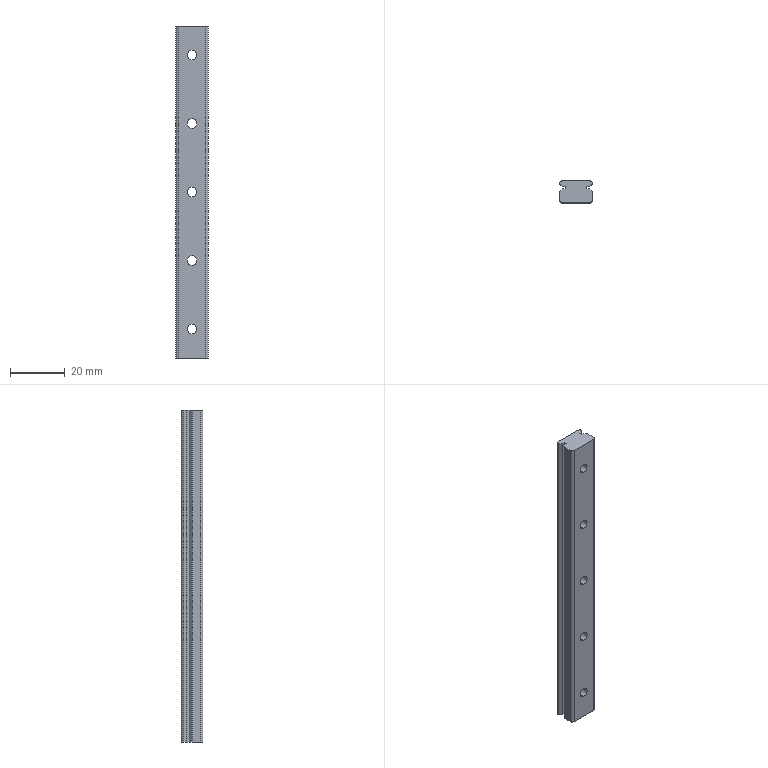Part | SolidWorks | features ICE 2, Extrusion 1 | 1 solid | 45 faces | box 12 x 8 x 121 mm | volume 9982 mm3 | cylinder 24 | plane 21 | commonest cylinder face diameters 3.5 x10 6 x10 2 x4
STEP:
#1=CARTESIAN_POINT('',(0.,-4.,108.75));
#2=VERTEX_POINT('',#1);
#3=CARTESIAN_POINT('',(0.,-4.,112.25));
#4=VERTEX_POINT('',#3);
#5=CARTESIAN_POINT('',(0.,-4.,110.5));
#6=DIRECTION('',(0.,1.,0.));
#7=DIRECTION('',(0.,0.,1.));
#8=AXIS2_PLACEMENT_3D('',#5,#6,#7);
#9=CIRCLE('',#8,1.75);
#10=EDGE_CURVE('',#2,#4,#9,.T.);
#11=ORIENTED_EDGE('',*,*,#10,.F.);
#12=CARTESIAN_POINT('',(0.,-0.5,108.75));
#13=VERTEX_POINT('',#12);
#14=CARTESIAN_POINT('',(0.,-4.,108.75));
#15=DIRECTION('',(0.,1.,0.));
#16=VECTOR('',#15,1000.);
#17=LINE('',#14,#16);
#18=EDGE_CURVE('',#2,#13,#17,.T.);
#19=ORIENTED_EDGE('',*,*,#18,.T.);
#20=CARTESIAN_POINT('',(0.,-0.5,112.25));
#21=VERTEX_POINT('',#20);
#22=CARTESIAN_POINT('',(0.,-0.5,110.5));
#23=DIRECTION('',(0.,1.,0.));
#24=DIRECTION('',(0.,0.,1.));
#25=AXIS2_PLACEMENT_3D('',#22,#23,#24);
#26=CIRCLE('',#25,1.75);
#27=EDGE_CURVE('',#13,#21,#26,.T.);
#28=ORIENTED_EDGE('',*,*,#27,.T.);
#29=CARTESIAN_POINT('',(0.,-4.,112.25));
#30=DIRECTION('',(0.,1.,0.));
#31=VECTOR('',#30,1000.);
#32=LINE('',#29,#31);
#33=EDGE_CURVE('',#4,#21,#32,.T.);
#34=ORIENTED_EDGE('',*,*,#33,.F.);
#35=EDGE_LOOP('',(#11,#19,#28,#34));
#36=FACE_OUTER_BOUND('',#35,.T.);
#37=CARTESIAN_POINT('',(0.,-4.,110.5));
#38=DIRECTION('',(0.,1.,0.));
#39=DIRECTION('',(0.,0.,1.));
#40=AXIS2_PLACEMENT_3D('',#37,#38,#39);
#41=CYLINDRICAL_SURFACE('',#40,1.75);
#42=ADVANCED_FACE('',(#36),#41,.F.);
#43=CARTESIAN_POINT('',(0.,-4.,83.75));
#44=VERTEX_POINT('',#43);
#45=CARTESIAN_POINT('',(0.,-4.,87.25));
#46=VERTEX_POINT('',#45);
#47=CARTESIAN_POINT('',(0.,-4.,85.5));
#48=DIRECTION('',(0.,1.,0.));
#49=DIRECTION('',(0.,0.,1.));
#50=AXIS2_PLACEMENT_3D('',#47,#48,#49);
#51=CIRCLE('',#50,1.75);
#52=EDGE_CURVE('',#44,#46,#51,.T.);
#53=ORIENTED_EDGE('',*,*,#52,.F.);
#54=CARTESIAN_POINT('',(0.,-0.5,83.75));
#55=VERTEX_POINT('',#54);
#56=CARTESIAN_POINT('',(0.,-4.,83.75));
#57=DIRECTION('',(0.,1.,0.));
#58=VECTOR('',#57,1000.);
#59=LINE('',#56,#58);
#60=EDGE_CURVE('',#44,#55,#59,.T.);
#61=ORIENTED_EDGE('',*,*,#60,.T.);
#62=CARTESIAN_POINT('',(0.,-0.5,87.25));
#63=VERTEX_POINT('',#62);
#64=CARTESIAN_POINT('',(0.,-0.5,85.5));
#65=DIRECTION('',(0.,1.,0.));
#66=DIRECTION('',(0.,0.,1.));
#67=AXIS2_PLACEMENT_3D('',#64,#65,#66);
#68=CIRCLE('',#67,1.75);
#69=EDGE_CURVE('',#55,#63,#68,.T.);
#70=ORIENTED_EDGE('',*,*,#69,.T.);
#71=CARTESIAN_POINT('',(0.,-4.,87.25));
#72=DIRECTION('',(0.,1.,0.));
#73=VECTOR('',#72,1000.);
#74=LINE('',#71,#73);
#75=EDGE_CURVE('',#46,#63,#74,.T.);
#76=ORIENTED_EDGE('',*,*,#75,.F.);
#77=EDGE_LOOP('',(#53,#61,#70,#76));
#78=FACE_OUTER_BOUND('',#77,.T.);
#79=CARTESIAN_POINT('',(0.,-4.,85.5));
#80=DIRECTION('',(0.,1.,0.));
#81=DIRECTION('',(0.,0.,1.));
#82=AXIS2_PLACEMENT_3D('',#79,#80,#81);
#83=CYLINDRICAL_SURFACE('',#82,1.75);
#84=ADVANCED_FACE('',(#78),#83,.F.);
#85=CARTESIAN_POINT('',(0.,-4.,58.75));
#86=VERTEX_POINT('',#85);
#87=CARTESIAN_POINT('',(0.,-4.,62.25));
#88=VERTEX_POINT('',#87);
#89=CARTESIAN_POINT('',(0.,-4.,60.5));
#90=DIRECTION('',(0.,1.,0.));
#91=DIRECTION('',(0.,0.,1.));
#92=AXIS2_PLACEMENT_3D('',#89,#90,#91);
#93=CIRCLE('',#92,1.75);
#94=EDGE_CURVE('',#86,#88,#93,.T.);
#95=ORIENTED_EDGE('',*,*,#94,.F.);
#96=CARTESIAN_POINT('',(0.,-0.5,58.75));
#97=VERTEX_POINT('',#96);
#98=CARTESIAN_POINT('',(0.,-4.,58.75));
#99=DIRECTION('',(0.,1.,0.));
#100=VECTOR('',#99,1000.);
#101=LINE('',#98,#100);
#102=EDGE_CURVE('',#86,#97,#101,.T.);
#103=ORIENTED_EDGE('',*,*,#102,.T.);
#104=CARTESIAN_POINT('',(0.,-0.5,62.25));
#105=VERTEX_POINT('',#104);
#106=CARTESIAN_POINT('',(0.,-0.5,60.5));
#107=DIRECTION('',(0.,1.,0.));
#108=DIRECTION('',(0.,0.,1.));
#109=AXIS2_PLACEMENT_3D('',#106,#107,#108);
#110=CIRCLE('',#109,1.75);
#111=EDGE_CURVE('',#97,#105,#110,.T.);
#112=ORIENTED_EDGE('',*,*,#111,.T.);
#113=CARTESIAN_POINT('',(0.,-4.,62.25));
#114=DIRECTION('',(0.,1.,0.));
#115=VECTOR('',#114,1000.);
#116=LINE('',#113,#115);
#117=EDGE_CURVE('',#88,#105,#116,.T.);
#118=ORIENTED_EDGE('',*,*,#117,.F.);
#119=EDGE_LOOP('',(#95,#103,#112,#118));
#120=FACE_OUTER_BOUND('',#119,.T.);
#121=CARTESIAN_POINT('',(0.,-4.,60.5));
#122=DIRECTION('',(0.,1.,0.));
#123=DIRECTION('',(0.,0.,1.));
#124=AXIS2_PLACEMENT_3D('',#121,#122,#123);
#125=CYLINDRICAL_SURFACE('',#124,1.75);
#126=ADVANCED_FACE('',(#120),#125,.F.);
#127=CARTESIAN_POINT('',(0.,-4.,8.75));
#128=VERTEX_POINT('',#127);
#129=CARTESIAN_POINT('',(0.,-4.,12.25));
#130=VERTEX_POINT('',#129);
#131=CARTESIAN_POINT('',(0.,-4.,10.5));
#132=DIRECTION('',(0.,1.,0.));
#133=DIRECTION('',(0.,0.,1.));
#134=AXIS2_PLACEMENT_3D('',#131,#132,#133);
#135=CIRCLE('',#134,1.75);
#136=EDGE_CURVE('',#128,#130,#135,.T.);
#137=ORIENTED_EDGE('',*,*,#136,.F.);
#138=CARTESIAN_POINT('',(0.,-0.5,8.75));
#139=VERTEX_POINT('',#138);
#140=CARTESIAN_POINT('',(0.,-4.,8.75));
#141=DIRECTION('',(0.,1.,0.));
#142=VECTOR('',#141,1000.);
#143=LINE('',#140,#142);
#144=EDGE_CURVE('',#128,#139,#143,.T.);
#145=ORIENTED_EDGE('',*,*,#144,.T.);
#146=CARTESIAN_POINT('',(0.,-0.5,12.25));
#147=VERTEX_POINT('',#146);
#148=CARTESIAN_POINT('',(0.,-0.5,10.5));
#149=DIRECTION('',(0.,1.,0.));
#150=DIRECTION('',(0.,0.,1.));
#151=AXIS2_PLACEMENT_3D('',#148,#149,#150);
#152=CIRCLE('',#151,1.75);
#153=EDGE_CURVE('',#139,#147,#152,.T.);
#154=ORIENTED_EDGE('',*,*,#153,.T.);
#155=CARTESIAN_POINT('',(0.,-4.,12.25));
#156=DIRECTION('',(0.,1.,0.));
#157=VECTOR('',#156,1000.);
#158=LINE('',#155,#157);
#159=EDGE_CURVE('',#130,#147,#158,.T.);
#160=ORIENTED_EDGE('',*,*,#159,.F.);
#161=EDGE_LOOP('',(#137,#145,#154,#160));
#162=FACE_OUTER_BOUND('',#161,.T.);
#163=CARTESIAN_POINT('',(0.,-4.,10.5));
#164=DIRECTION('',(0.,1.,0.));
#165=DIRECTION('',(0.,0.,1.));
#166=AXIS2_PLACEMENT_3D('',#163,#164,#165);
#167=CYLINDRICAL_SURFACE('',#166,1.75);
#168=ADVANCED_FACE('',(#162),#167,.F.);
#169=CARTESIAN_POINT('',(0.,-4.,33.75));
#170=VERTEX_POINT('',#169);
#171=CARTESIAN_POINT('',(0.,-4.,37.25));
#172=VERTEX_POINT('',#171);
#173=CARTESIAN_POINT('',(0.,-4.,35.5));
#174=DIRECTION('',(0.,1.,0.));
#175=DIRECTION('',(0.,0.,1.));
#176=AXIS2_PLACEMENT_3D('',#173,#174,#175);
#177=CIRCLE('',#176,1.75);
#178=EDGE_CURVE('',#170,#172,#177,.T.);
#179=ORIENTED_EDGE('',*,*,#178,.F.);
#180=CARTESIAN_POINT('',(0.,-0.5,33.75));
#181=VERTEX_POINT('',#180);
#182=CARTESIAN_POINT('',(0.,-4.,33.75));
#183=DIRECTION('',(0.,1.,0.));
#184=VECTOR('',#183,1000.);
#185=LINE('',#182,#184);
#186=EDGE_CURVE('',#170,#181,#185,.T.);
#187=ORIENTED_EDGE('',*,*,#186,.T.);
#188=CARTESIAN_POINT('',(0.,-0.5,37.25));
#189=VERTEX_POINT('',#188);
#190=CARTESIAN_POINT('',(0.,-0.5,35.5));
#191=DIRECTION('',(0.,1.,0.));
#192=DIRECTION('',(0.,0.,1.));
#193=AXIS2_PLACEMENT_3D('',#190,#191,#192);
#194=CIRCLE('',#193,1.75);
#195=EDGE_CURVE('',#181,#189,#194,.T.);
#196=ORIENTED_EDGE('',*,*,#195,.T.);
#197=CARTESIAN_POINT('',(0.,-4.,37.25));
#198=DIRECTION('',(0.,1.,0.));
#199=VECTOR('',#198,1000.);
#200=LINE('',#197,#199);
#201=EDGE_CURVE('',#172,#189,#200,.T.);
#202=ORIENTED_EDGE('',*,*,#201,.F.);
#203=EDGE_LOOP('',(#179,#187,#196,#202));
#204=FACE_OUTER_BOUND('',#203,.T.);
#205=CARTESIAN_POINT('',(0.,-4.,35.5));
#206=DIRECTION('',(0.,1.,0.));
#207=DIRECTION('',(0.,0.,1.));
#208=AXIS2_PLACEMENT_3D('',#205,#206,#207);
#209=CYLINDRICAL_SURFACE('',#208,1.75);
#210=ADVANCED_FACE('',(#204),#209,.F.);
#211=CARTESIAN_POINT('',(0.,-0.5,107.5));
#212=VERTEX_POINT('',#211);
#213=CARTESIAN_POINT('',(0.,-0.5,113.5));
#214=VERTEX_POINT('',#213);
#215=CARTESIAN_POINT('',(0.,-0.5,110.5));
#216=DIRECTION('',(0.,1.,0.));
#217=DIRECTION('',(0.,0.,1.));
#218=AXIS2_PLACEMENT_3D('',#215,#216,#217);
#219=CIRCLE('',#218,3.);
#220=EDGE_CURVE('',#212,#214,#219,.T.);
#221=ORIENTED_EDGE('',*,*,#220,.F.);
#222=CARTESIAN_POINT('',(0.,4.,107.5));
#223=VERTEX_POINT('',#222);
#224=CARTESIAN_POINT('',(0.,-0.5,107.5));
#225=DIRECTION('',(0.,1.,0.));
#226=VECTOR('',#225,1000.);
#227=LINE('',#224,#226);
#228=EDGE_CURVE('',#212,#223,#227,.T.);
#229=ORIENTED_EDGE('',*,*,#228,.T.);
#230=CARTESIAN_POINT('',(0.,4.,113.5));
#231=VERTEX_POINT('',#230);
#232=CARTESIAN_POINT('',(0.,4.,110.5));
#233=DIRECTION('',(0.,1.,0.));
#234=DIRECTION('',(0.,0.,1.));
#235=AXIS2_PLACEMENT_3D('',#232,#233,#234);
#236=CIRCLE('',#235,3.);
#237=EDGE_CURVE('',#223,#231,#236,.T.);
#238=ORIENTED_EDGE('',*,*,#237,.T.);
#239=CARTESIAN_POINT('',(0.,-0.5,113.5));
#240=DIRECTION('',(0.,1.,0.));
#241=VECTOR('',#240,1000.);
#242=LINE('',#239,#241);
#243=EDGE_CURVE('',#214,#231,#242,.T.);
#244=ORIENTED_EDGE('',*,*,#243,.F.);
#245=EDGE_LOOP('',(#221,#229,#238,#244));
#246=FACE_OUTER_BOUND('',#245,.T.);
#247=CARTESIAN_POINT('',(0.,-0.5,110.5));
#248=DIRECTION('',(0.,1.,0.));
#249=DIRECTION('',(0.,0.,1.));
#250=AXIS2_PLACEMENT_3D('',#247,#248,#249);
#251=CYLINDRICAL_SURFACE('',#250,3.);
#252=ADVANCED_FACE('',(#246),#251,.F.);
#253=CARTESIAN_POINT('',(0.,-0.5,82.5));
#254=VERTEX_POINT('',#253);
#255=CARTESIAN_POINT('',(0.,-0.5,88.5));
#256=VERTEX_POINT('',#255);
#257=CARTESIAN_POINT('',(0.,-0.5,85.5));
#258=DIRECTION('',(0.,1.,0.));
#259=DIRECTION('',(0.,0.,1.));
#260=AXIS2_PLACEMENT_3D('',#257,#258,#259);
#261=CIRCLE('',#260,3.);
#262=EDGE_CURVE('',#254,#256,#261,.T.);
#263=ORIENTED_EDGE('',*,*,#262,.F.);
#264=CARTESIAN_POINT('',(0.,4.,82.5));
#265=VERTEX_POINT('',#264);
#266=CARTESIAN_POINT('',(0.,-0.5,82.5));
#267=DIRECTION('',(0.,1.,0.));
#268=VECTOR('',#267,1000.);
#269=LINE('',#266,#268);
#270=EDGE_CURVE('',#254,#265,#269,.T.);
#271=ORIENTED_EDGE('',*,*,#270,.T.);
#272=CARTESIAN_POINT('',(0.,4.,88.5));
#273=VERTEX_POINT('',#272);
#274=CARTESIAN_POINT('',(0.,4.,85.5));
#275=DIRECTION('',(0.,1.,0.));
#276=DIRECTION('',(0.,0.,1.));
#277=AXIS2_PLACEMENT_3D('',#274,#275,#276);
#278=CIRCLE('',#277,3.);
#279=EDGE_CURVE('',#265,#273,#278,.T.);
#280=ORIENTED_EDGE('',*,*,#279,.T.);
#281=CARTESIAN_POINT('',(0.,-0.5,88.5));
#282=DIRECTION('',(0.,1.,0.));
#283=VECTOR('',#282,1000.);
#284=LINE('',#281,#283);
#285=EDGE_CURVE('',#256,#273,#284,.T.);
#286=ORIENTED_EDGE('',*,*,#285,.F.);
#287=EDGE_LOOP('',(#263,#271,#280,#286));
#288=FACE_OUTER_BOUND('',#287,.T.);
#289=CARTESIAN_POINT('',(0.,-0.5,85.5));
#290=DIRECTION('',(0.,1.,0.));
#291=DIRECTION('',(0.,0.,1.));
#292=AXIS2_PLACEMENT_3D('',#289,#290,#291);
#293=CYLINDRICAL_SURFACE('',#292,3.);
#294=ADVANCED_FACE('',(#288),#293,.F.);
#295=CARTESIAN_POINT('',(0.,-0.5,57.5));
#296=VERTEX_POINT('',#295);
#297=CARTESIAN_POINT('',(0.,-0.5,63.5));
#298=VERTEX_POINT('',#297);
#299=CARTESIAN_POINT('',(0.,-0.5,60.5));
#300=DIRECTION('',(0.,1.,0.));
#301=DIRECTION('',(0.,0.,1.));
#302=AXIS2_PLACEMENT_3D('',#299,#300,#301);
#303=CIRCLE('',#302,3.);
#304=EDGE_CURVE('',#296,#298,#303,.T.);
#305=ORIENTED_EDGE('',*,*,#304,.F.);
#306=CARTESIAN_POINT('',(0.,4.,57.5));
#307=VERTEX_POINT('',#306);
#308=CARTESIAN_POINT('',(0.,-0.5,57.5));
#309=DIRECTION('',(0.,1.,0.));
#310=VECTOR('',#309,1000.);
#311=LINE('',#308,#310);
#312=EDGE_CURVE('',#296,#307,#311,.T.);
#313=ORIENTED_EDGE('',*,*,#312,.T.);
#314=CARTESIAN_POINT('',(0.,4.,63.5));
#315=VERTEX_POINT('',#314);
#316=CARTESIAN_POINT('',(0.,4.,60.5));
#317=DIRECTION('',(0.,1.,0.));
#318=DIRECTION('',(0.,0.,1.));
#319=AXIS2_PLACEMENT_3D('',#316,#317,#318);
#320=CIRCLE('',#319,3.);
#321=EDGE_CURVE('',#307,#315,#320,.T.);
#322=ORIENTED_EDGE('',*,*,#321,.T.);
#323=CARTESIAN_POINT('',(0.,-0.5,63.5));
#324=DIRECTION('',(0.,1.,0.));
#325=VECTOR('',#324,1000.);
#326=LINE('',#323,#325);
#327=EDGE_CURVE('',#298,#315,#326,.T.);
#328=ORIENTED_EDGE('',*,*,#327,.F.);
#329=EDGE_LOOP('',(#305,#313,#322,#328));
#330=FACE_OUTER_BOUND('',#329,.T.);
#331=CARTESIAN_POINT('',(0.,-0.5,60.5));
#332=DIRECTION('',(0.,1.,0.));
#333=DIRECTION('',(0.,0.,1.));
#334=AXIS2_PLACEMENT_3D('',#331,#332,#333);
#335=CYLINDRICAL_SURFACE('',#334,3.);
#336=ADVANCED_FACE('',(#330),#335,.F.);
#337=CARTESIAN_POINT('',(0.,-0.5,32.5));
#338=VERTEX_POINT('',#337);
#339=CARTESIAN_POINT('',(0.,-0.5,38.5));
#340=VERTEX_POINT('',#339);
#341=CARTESIAN_POINT('',(0.,-0.5,35.5));
#342=DIRECTION('',(0.,1.,0.));
#343=DIRECTION('',(0.,0.,1.));
#344=AXIS2_PLACEMENT_3D('',#341,#342,#343);
#345=CIRCLE('',#344,3.);
#346=EDGE_CURVE('',#338,#340,#345,.T.);
#347=ORIENTED_EDGE('',*,*,#346,.F.);
#348=CARTESIAN_POINT('',(0.,4.,32.5));
#349=VERTEX_POINT('',#348);
#350=CARTESIAN_POINT('',(0.,-0.5,32.5));
#351=DIRECTION('',(0.,1.,0.));
#352=VECTOR('',#351,1000.);
#353=LINE('',#350,#352);
#354=EDGE_CURVE('',#338,#349,#353,.T.);
#355=ORIENTED_EDGE('',*,*,#354,.T.);
#356=CARTESIAN_POINT('',(0.,4.,38.5));
#357=VERTEX_POINT('',#356);
#358=CARTESIAN_POINT('',(0.,4.,35.5));
#359=DIRECTION('',(0.,1.,0.));
#360=DIRECTION('',(0.,0.,1.));
#361=AXIS2_PLACEMENT_3D('',#358,#359,#360);
#362=CIRCLE('',#361,3.);
#363=EDGE_CURVE('',#349,#357,#362,.T.);
#364=ORIENTED_EDGE('',*,*,#363,.T.);
#365=CARTESIAN_POINT('',(0.,-0.5,38.5));
#366=DIRECTION('',(0.,1.,0.));
#367=VECTOR('',#366,1000.);
#368=LINE('',#365,#367);
#369=EDGE_CURVE('',#340,#357,#368,.T.);
#370=ORIENTED_EDGE('',*,*,#369,.F.);
#371=EDGE_LOOP('',(#347,#355,#364,#370));
#372=FACE_OUTER_BOUND('',#371,.T.);
#373=CARTESIAN_POINT('',(0.,-0.5,35.5));
#374=DIRECTION('',(0.,1.,0.));
#375=DIRECTION('',(0.,0.,1.));
#376=AXIS2_PLACEMENT_3D('',#373,#374,#375);
#377=CYLINDRICAL_SURFACE('',#376,3.);
#378=ADVANCED_FACE('',(#372),#377,.F.);
#379=CARTESIAN_POINT('',(0.,-0.5,7.5));
#380=VERTEX_POINT('',#379);
#381=CARTESIAN_POINT('',(0.,-0.5,13.5));
#382=VERTEX_POINT('',#381);
#383=CARTESIAN_POINT('',(0.,-0.5,10.5));
#384=DIRECTION('',(0.,1.,0.));
#385=DIRECTION('',(0.,0.,1.));
#386=AXIS2_PLACEMENT_3D('',#383,#384,#385);
#387=CIRCLE('',#386,3.);
#388=EDGE_CURVE('',#380,#382,#387,.T.);
#389=ORIENTED_EDGE('',*,*,#388,.F.);
#390=CARTESIAN_POINT('',(0.,4.,7.5));
#391=VERTEX_POINT('',#390);
#392=CARTESIAN_POINT('',(0.,-0.5,7.5));
#393=DIRECTION('',(0.,1.,0.));
#394=VECTOR('',#393,1000.);
#395=LINE('',#392,#394);
#396=EDGE_CURVE('',#380,#391,#395,.T.);
#397=ORIENTED_EDGE('',*,*,#396,.T.);
#398=CARTESIAN_POINT('',(0.,4.,13.5));
#399=VERTEX_POINT('',#398);
#400=CARTESIAN_POINT('',(0.,4.,10.5));
#401=DIRECTION('',(0.,1.,0.));
#402=DIRECTION('',(0.,0.,1.));
#403=AXIS2_PLACEMENT_3D('',#400,#401,#402);
#404=CIRCLE('',#403,3.);
#405=EDGE_CURVE('',#391,#399,#404,.T.);
#406=ORIENTED_EDGE('',*,*,#405,.T.);
#407=CARTESIAN_POINT('',(0.,-0.5,13.5));
#408=DIRECTION('',(0.,1.,0.));
#409=VECTOR('',#408,1000.);
#410=LINE('',#407,#409);
#411=EDGE_CURVE('',#382,#399,#410,.T.);
#412=ORIENTED_EDGE('',*,*,#411,.F.);
#413=EDGE_LOOP('',(#389,#397,#406,#412));
#414=FACE_OUTER_BOUND('',#413,.T.);
#415=CARTESIAN_POINT('',(0.,-0.5,10.5));
#416=DIRECTION('',(0.,1.,0.));
#417=DIRECTION('',(0.,0.,1.));
#418=AXIS2_PLACEMENT_3D('',#415,#416,#417);
#419=CYLINDRICAL_SURFACE('',#418,3.);
#420=ADVANCED_FACE('',(#414),#419,.F.);
#421=CARTESIAN_POINT('',(-6.,-3.,0.));
#422=VERTEX_POINT('',#421);
#423=CARTESIAN_POINT('',(-5.,-4.,0.));
#424=VERTEX_POINT('',#423);
#425=CARTESIAN_POINT('',(-5.,-3.,0.));
#426=DIRECTION('',(0.,0.,1.));
#427=DIRECTION('',(1.,0.,0.));
#428=AXIS2_PLACEMENT_3D('',#425,#426,#427);
#429=CIRCLE('',#428,1.);
#430=EDGE_CURVE('',#422,#424,#429,.T.);
#431=ORIENTED_EDGE('',*,*,#430,.T.);
#432=CARTESIAN_POINT('',(-5.,-4.,121.));
#433=VERTEX_POINT('',#432);
#434=CARTESIAN_POINT('',(-5.,-4.,121.));
#435=DIRECTION('',(0.,0.,-1.));
#436=VECTOR('',#435,1000.);
#437=LINE('',#434,#436);
#438=EDGE_CURVE('',#433,#424,#437,.T.);
#439=ORIENTED_EDGE('',*,*,#438,.F.);
#440=CARTESIAN_POINT('',(-6.,-3.,121.));
#441=VERTEX_POINT('',#440);
#442=CARTESIAN_POINT('',(-5.,-3.,121.));
#443=DIRECTION('',(0.,0.,1.));
#444=DIRECTION('',(1.,0.,0.));
#445=AXIS2_PLACEMENT_3D('',#442,#443,#444);
#446=CIRCLE('',#445,1.);
#447=EDGE_CURVE('',#441,#433,#446,.T.);
#448=ORIENTED_EDGE('',*,*,#447,.F.);
#449=CARTESIAN_POINT('',(-6.,-3.,121.));
#450=DIRECTION('',(0.,0.,-1.));
#451=VECTOR('',#450,1000.);
#452=LINE('',#449,#451);
#453=EDGE_CURVE('',#441,#422,#452,.T.);
#454=ORIENTED_EDGE('',*,*,#453,.T.);
#455=EDGE_LOOP('',(#431,#439,#448,#454));
#456=FACE_OUTER_BOUND('',#455,.T.);
#457=CARTESIAN_POINT('',(-5.,-3.,121.));
#458=DIRECTION('',(0.,0.,-1.));
#459=DIRECTION('',(-1.,0.,0.));
#460=AXIS2_PLACEMENT_3D('',#457,#458,#459);
#461=CYLINDRICAL_SURFACE('',#460,1.);
#462=ADVANCED_FACE('',(#456),#461,.T.);
#463=CARTESIAN_POINT('',(0.,-4.,110.5));
#464=DIRECTION('',(0.,1.,0.));
#465=DIRECTION('',(0.,0.,1.));
#466=AXIS2_PLACEMENT_3D('',#463,#464,#465);
#467=CIRCLE('',#466,1.75);
#468=EDGE_CURVE('',#4,#2,#467,.T.);
#469=ORIENTED_EDGE('',*,*,#468,.T.);
#470=ORIENTED_EDGE('',*,*,#10,.T.);
#471=EDGE_LOOP('',(#469,#470));
#472=FACE_BOUND('',#471,.T.);
#473=CARTESIAN_POINT('',(0.,-4.,85.5));
#474=DIRECTION('',(0.,1.,0.));
#475=DIRECTION('',(0.,0.,1.));
#476=AXIS2_PLACEMENT_3D('',#473,#474,#475);
#477=CIRCLE('',#476,1.75);
#478=EDGE_CURVE('',#46,#44,#477,.T.);
#479=ORIENTED_EDGE('',*,*,#478,.T.);
#480=ORIENTED_EDGE('',*,*,#52,.T.);
#481=EDGE_LOOP('',(#479,#480));
#482=FACE_BOUND('',#481,.T.);
#483=CARTESIAN_POINT('',(0.,-4.,60.5));
#484=DIRECTION('',(0.,1.,0.));
#485=DIRECTION('',(0.,0.,1.));
#486=AXIS2_PLACEMENT_3D('',#483,#484,#485);
#487=CIRCLE('',#486,1.75);
#488=EDGE_CURVE('',#88,#86,#487,.T.);
#489=ORIENTED_EDGE('',*,*,#488,.T.);
#490=ORIENTED_EDGE('',*,*,#94,.T.);
#491=EDGE_LOOP('',(#489,#490));
#492=FACE_BOUND('',#491,.T.);
#493=CARTESIAN_POINT('',(0.,-4.,10.5));
#494=DIRECTION('',(0.,1.,0.));
#495=DIRECTION('',(0.,0.,1.));
#496=AXIS2_PLACEMENT_3D('',#493,#494,#495);
#497=CIRCLE('',#496,1.75);
#498=EDGE_CURVE('',#130,#128,#497,.T.);
#499=ORIENTED_EDGE('',*,*,#498,.T.);
#500=ORIENTED_EDGE('',*,*,#136,.T.);
#501=EDGE_LOOP('',(#499,#500));
#502=FACE_BOUND('',#501,.T.);
#503=CARTESIAN_POINT('',(0.,-4.,35.5));
#504=DIRECTION('',(0.,1.,0.));
#505=DIRECTION('',(0.,0.,1.));
#506=AXIS2_PLACEMENT_3D('',#503,#504,#505);
#507=CIRCLE('',#506,1.75);
#508=EDGE_CURVE('',#172,#170,#507,.T.);
#509=ORIENTED_EDGE('',*,*,#508,.T.);
#510=ORIENTED_EDGE('',*,*,#178,.T.);
#511=EDGE_LOOP('',(#509,#510));
#512=FACE_BOUND('',#511,.T.);
#513=CARTESIAN_POINT('',(5.,-4.,0.));
#514=VERTEX_POINT('',#513);
#515=CARTESIAN_POINT('',(-5.,-4.,0.));
#516=DIRECTION('',(1.,0.,0.));
#517=VECTOR('',#516,1000.);
#518=LINE('',#515,#517);
#519=EDGE_CURVE('',#424,#514,#518,.T.);
#520=ORIENTED_EDGE('',*,*,#519,.T.);
#521=CARTESIAN_POINT('',(5.,-4.,121.));
#522=VERTEX_POINT('',#521);
#523=CARTESIAN_POINT('',(5.,-4.,121.));
#524=DIRECTION('',(0.,0.,-1.));
#525=VECTOR('',#524,1000.);
#526=LINE('',#523,#525);
#527=EDGE_CURVE('',#522,#514,#526,.T.);
#528=ORIENTED_EDGE('',*,*,#527,.F.);
#529=CARTESIAN_POINT('',(-5.,-4.,121.));
#530=DIRECTION('',(1.,0.,0.));
#531=VECTOR('',#530,1000.);
#532=LINE('',#529,#531);
#533=EDGE_CURVE('',#433,#522,#532,.T.);
#534=ORIENTED_EDGE('',*,*,#533,.F.);
#535=ORIENTED_EDGE('',*,*,#438,.T.);
#536=EDGE_LOOP('',(#520,#528,#534,#535));
#537=FACE_OUTER_BOUND('',#536,.T.);
#538=CARTESIAN_POINT('',(-5.,-4.,121.));
#539=DIRECTION('',(0.,1.,0.));
#540=DIRECTION('',(0.,0.,1.));
#541=AXIS2_PLACEMENT_3D('',#538,#539,#540);
#542=PLANE('',#541);
#543=ADVANCED_FACE('',(#472,#482,#492,#502,#512,#537),#542,.F.);
#544=CARTESIAN_POINT('',(6.,-3.,0.));
#545=VERTEX_POINT('',#544);
#546=CARTESIAN_POINT('',(5.,-3.,0.));
#547=DIRECTION('',(0.,0.,1.));
#548=DIRECTION('',(1.,0.,0.));
#549=AXIS2_PLACEMENT_3D('',#546,#547,#548);
#550=CIRCLE('',#549,1.);
#551=EDGE_CURVE('',#514,#545,#550,.T.);
#552=ORIENTED_EDGE('',*,*,#551,.T.);
#553=CARTESIAN_POINT('',(6.,-3.,121.));
#554=VERTEX_POINT('',#553);
#555=CARTESIAN_POINT('',(6.,-3.,121.));
#556=DIRECTION('',(0.,0.,-1.));
#557=VECTOR('',#556,1000.);
#558=LINE('',#555,#557);
#559=EDGE_CURVE('',#554,#545,#558,.T.);
#560=ORIENTED_EDGE('',*,*,#559,.F.);
#561=CARTESIAN_POINT('',(5.,-3.,121.));
#562=DIRECTION('',(0.,0.,1.));
#563=DIRECTION('',(1.,0.,0.));
#564=AXIS2_PLACEMENT_3D('',#561,#562,#563);
#565=CIRCLE('',#564,1.);
#566=EDGE_CURVE('',#522,#554,#565,.T.);
#567=ORIENTED_EDGE('',*,*,#566,.F.);
#568=ORIENTED_EDGE('',*,*,#527,.T.);
#569=EDGE_LOOP('',(#552,#560,#567,#568));
#570=FACE_OUTER_BOUND('',#569,.T.);
#571=CARTESIAN_POINT('',(5.,-3.,121.));
#572=DIRECTION('',(0.,0.,-1.));
#573=DIRECTION('',(-1.,0.,0.));
#574=AXIS2_PLACEMENT_3D('',#571,#572,#573);
#575=CYLINDRICAL_SURFACE('',#574,1.);
#576=ADVANCED_FACE('',(#570),#575,.T.);
#577=CARTESIAN_POINT('',(6.,0.,0.));
#578=VERTEX_POINT('',#577);
#579=CARTESIAN_POINT('',(6.,0.,0.));
#580=DIRECTION('',(0.,1.,0.));
#581=VECTOR('',#580,1000.);
#582=LINE('',#579,#581);
#583=EDGE_CURVE('',#545,#578,#582,.T.);
#584=ORIENTED_EDGE('',*,*,#583,.T.);
#585=CARTESIAN_POINT('',(6.,0.,121.));
#586=VERTEX_POINT('',#585);
#587=CARTESIAN_POINT('',(6.,0.,121.));
#588=DIRECTION('',(0.,0.,-1.));
#589=VECTOR('',#588,1000.);
#590=LINE('',#587,#589);
#591=EDGE_CURVE('',#586,#578,#590,.T.);
#592=ORIENTED_EDGE('',*,*,#591,.F.);
#593=CARTESIAN_POINT('',(6.,0.,121.));
#594=DIRECTION('',(0.,1.,0.));
#595=VECTOR('',#594,1000.);
#596=LINE('',#593,#595);
#597=EDGE_CURVE('',#554,#586,#596,.T.);
#598=ORIENTED_EDGE('',*,*,#597,.F.);
#599=ORIENTED_EDGE('',*,*,#559,.T.);
#600=EDGE_LOOP('',(#584,#592,#598,#599));
#601=FACE_OUTER_BOUND('',#600,.T.);
#602=CARTESIAN_POINT('',(6.,0.,121.));
#603=DIRECTION('',(-1.,0.,0.));
#604=DIRECTION('',(0.,-1.,0.));
#605=AXIS2_PLACEMENT_3D('',#602,#603,#604);
#606=PLANE('',#605);
#607=ADVANCED_FACE('',(#601),#606,.F.);
#608=CARTESIAN_POINT('',(5.,1.,0.));
#609=VERTEX_POINT('',#608);
#610=CARTESIAN_POINT('',(5.,1.,0.));
#611=DIRECTION('',(-0.7071,0.7071,0.));
#612=VECTOR('',#611,1000.);
#613=LINE('',#610,#612);
#614=EDGE_CURVE('',#578,#609,#613,.T.);
#615=ORIENTED_EDGE('',*,*,#614,.T.);
#616=CARTESIAN_POINT('',(5.,1.,121.));
#617=VERTEX_POINT('',#616);
#618=CARTESIAN_POINT('',(5.,1.,121.));
#619=DIRECTION('',(0.,0.,-1.));
#620=VECTOR('',#619,1000.);
#621=LINE('',#618,#620);
#622=EDGE_CURVE('',#617,#609,#621,.T.);
#623=ORIENTED_EDGE('',*,*,#622,.F.);
#624=CARTESIAN_POINT('',(5.,1.,121.));
#625=DIRECTION('',(-0.7071,0.7071,0.));
#626=VECTOR('',#625,1000.);
#627=LINE('',#624,#626);
#628=EDGE_CURVE('',#586,#617,#627,.T.);
#629=ORIENTED_EDGE('',*,*,#628,.F.);
#630=ORIENTED_EDGE('',*,*,#591,.T.);
#631=EDGE_LOOP('',(#615,#623,#629,#630));
#632=FACE_OUTER_BOUND('',#631,.T.);
#633=CARTESIAN_POINT('',(5.,1.,121.));
#634=DIRECTION('',(-0.7071,-0.7071,0.));
#635=DIRECTION('',(0.7071,-0.7071,0.));
#636=AXIS2_PLACEMENT_3D('',#633,#634,#635);
#637=PLANE('',#636);
#638=ADVANCED_FACE('',(#632),#637,.F.);
#639=CARTESIAN_POINT('',(4.,1.,0.));
#640=VERTEX_POINT('',#639);
#641=CARTESIAN_POINT('',(4.,1.,0.));
#642=DIRECTION('',(-1.,0.,0.));
#643=VECTOR('',#642,1000.);
#644=LINE('',#641,#643);
#645=EDGE_CURVE('',#609,#640,#644,.T.);
#646=ORIENTED_EDGE('',*,*,#645,.T.);
#647=CARTESIAN_POINT('',(4.,1.,121.));
#648=VERTEX_POINT('',#647);
#649=CARTESIAN_POINT('',(4.,1.,121.));
#650=DIRECTION('',(0.,0.,-1.));
#651=VECTOR('',#650,1000.);
#652=LINE('',#649,#651);
#653=EDGE_CURVE('',#648,#640,#652,.T.);
#654=ORIENTED_EDGE('',*,*,#653,.F.);
#655=CARTESIAN_POINT('',(4.,1.,121.));
#656=DIRECTION('',(-1.,0.,0.));
#657=VECTOR('',#656,1000.);
#658=LINE('',#655,#657);
#659=EDGE_CURVE('',#617,#648,#658,.T.);
#660=ORIENTED_EDGE('',*,*,#659,.F.);
#661=ORIENTED_EDGE('',*,*,#622,.T.);
#662=EDGE_LOOP('',(#646,#654,#660,#661));
#663=FACE_OUTER_BOUND('',#662,.T.);
#664=CARTESIAN_POINT('',(4.,1.,121.));
#665=DIRECTION('',(0.,-1.,0.));
#666=DIRECTION('',(0.,0.,-1.));
#667=AXIS2_PLACEMENT_3D('',#664,#665,#666);
#668=PLANE('',#667);
#669=ADVANCED_FACE('',(#663),#668,.F.);
#670=CARTESIAN_POINT('',(4.,2.,0.));
#671=VERTEX_POINT('',#670);
#672=CARTESIAN_POINT('',(4.,2.,0.));
#673=DIRECTION('',(0.,1.,0.));
#674=VECTOR('',#673,1000.);
#675=LINE('',#672,#674);
#676=EDGE_CURVE('',#640,#671,#675,.T.);
#677=ORIENTED_EDGE('',*,*,#676,.T.);
#678=CARTESIAN_POINT('',(4.,2.,121.));
#679=VERTEX_POINT('',#678);
#680=CARTESIAN_POINT('',(4.,2.,121.));
#681=DIRECTION('',(0.,0.,-1.));
#682=VECTOR('',#681,1000.);
#683=LINE('',#680,#682);
#684=EDGE_CURVE('',#679,#671,#683,.T.);
#685=ORIENTED_EDGE('',*,*,#684,.F.);
#686=CARTESIAN_POINT('',(4.,2.,121.));
#687=DIRECTION('',(0.,1.,0.));
#688=VECTOR('',#687,1000.);
#689=LINE('',#686,#688);
#690=EDGE_CURVE('',#648,#679,#689,.T.);
#691=ORIENTED_EDGE('',*,*,#690,.F.);
#692=ORIENTED_EDGE('',*,*,#653,.T.);
#693=EDGE_LOOP('',(#677,#685,#691,#692));
#694=FACE_OUTER_BOUND('',#693,.T.);
#695=CARTESIAN_POINT('',(4.,2.,121.));
#696=DIRECTION('',(-1.,0.,0.));
#697=DIRECTION('',(0.,0.,1.));
#698=AXIS2_PLACEMENT_3D('',#695,#696,#697);
#699=PLANE('',#698);
#700=ADVANCED_FACE('',(#694),#699,.F.);
#701=CARTESIAN_POINT('',(5.,2.,0.));
#702=VERTEX_POINT('',#701);
#703=CARTESIAN_POINT('',(5.,2.,0.));
#704=DIRECTION('',(1.,0.,0.));
#705=VECTOR('',#704,1000.);
#706=LINE('',#703,#705);
#707=EDGE_CURVE('',#671,#702,#706,.T.);
#708=ORIENTED_EDGE('',*,*,#707,.T.);
#709=CARTESIAN_POINT('',(5.,2.,121.));
#710=VERTEX_POINT('',#709);
#711=CARTESIAN_POINT('',(5.,2.,121.));
#712=DIRECTION('',(0.,0.,-1.));
#713=VECTOR('',#712,1000.);
#714=LINE('',#711,#713);
#715=EDGE_CURVE('',#710,#702,#714,.T.);
#716=ORIENTED_EDGE('',*,*,#715,.F.);
#717=CARTESIAN_POINT('',(5.,2.,121.));
#718=DIRECTION('',(1.,0.,0.));
#719=VECTOR('',#718,1000.);
#720=LINE('',#717,#719);
#721=EDGE_CURVE('',#679,#710,#720,.T.);
#722=ORIENTED_EDGE('',*,*,#721,.F.);
#723=ORIENTED_EDGE('',*,*,#684,.T.);
#724=EDGE_LOOP('',(#708,#716,#722,#723));
#725=FACE_OUTER_BOUND('',#724,.T.);
#726=CARTESIAN_POINT('',(5.,2.,121.));
#727=DIRECTION('',(0.,1.,0.));
#728=DIRECTION('',(0.,0.,1.));
#729=AXIS2_PLACEMENT_3D('',#726,#727,#728);
#730=PLANE('',#729);
#731=ADVANCED_FACE('',(#725),#730,.F.);
#732=CARTESIAN_POINT('',(6.,3.,0.));
#733=VERTEX_POINT('',#732);
#734=CARTESIAN_POINT('',(5.,2.,0.));
#735=DIRECTION('',(0.7071,0.7071,0.));
#736=VECTOR('',#735,1000.);
#737=LINE('',#734,#736);
#738=EDGE_CURVE('',#702,#733,#737,.T.);
#739=ORIENTED_EDGE('',*,*,#738,.T.);
#740=CARTESIAN_POINT('',(6.,3.,121.));
#741=VERTEX_POINT('',#740);
#742=CARTESIAN_POINT('',(6.,3.,121.));
#743=DIRECTION('',(0.,0.,-1.));
#744=VECTOR('',#743,1000.);
#745=LINE('',#742,#744);
#746=EDGE_CURVE('',#741,#733,#745,.T.);
#747=ORIENTED_EDGE('',*,*,#746,.F.);
#748=CARTESIAN_POINT('',(5.,2.,121.));
#749=DIRECTION('',(0.7071,0.7071,0.));
#750=VECTOR('',#749,1000.);
#751=LINE('',#748,#750);
#752=EDGE_CURVE('',#710,#741,#751,.T.);
#753=ORIENTED_EDGE('',*,*,#752,.F.);
#754=ORIENTED_EDGE('',*,*,#715,.T.);
#755=EDGE_LOOP('',(#739,#747,#753,#754));
#756=FACE_OUTER_BOUND('',#755,.T.);
#757=CARTESIAN_POINT('',(5.,2.,121.));
#758=DIRECTION('',(-0.7071,0.7071,0.));
#759=DIRECTION('',(-0.7071,-0.7071,0.));
#760=AXIS2_PLACEMENT_3D('',#757,#758,#759);
#761=PLANE('',#760);
#762=ADVANCED_FACE('',(#756),#761,.F.);
#763=CARTESIAN_POINT('',(5.,4.,0.));
#764=VERTEX_POINT('',#763);
#765=CARTESIAN_POINT('',(5.,3.,0.));
#766=DIRECTION('',(0.,0.,1.));
#767=DIRECTION('',(-1.,0.,0.));
#768=AXIS2_PLACEMENT_3D('',#765,#766,#767);
#769=CIRCLE('',#768,1.);
#770=EDGE_CURVE('',#733,#764,#769,.T.);
#771=ORIENTED_EDGE('',*,*,#770,.T.);
#772=CARTESIAN_POINT('',(5.,4.,121.));
#773=VERTEX_POINT('',#772);
#774=CARTESIAN_POINT('',(5.,4.,121.));
#775=DIRECTION('',(0.,0.,-1.));
#776=VECTOR('',#775,1000.);
#777=LINE('',#774,#776);
#778=EDGE_CURVE('',#773,#764,#777,.T.);
#779=ORIENTED_EDGE('',*,*,#778,.F.);
#780=CARTESIAN_POINT('',(5.,3.,121.));
#781=DIRECTION('',(0.,0.,1.));
#782=DIRECTION('',(-1.,0.,0.));
#783=AXIS2_PLACEMENT_3D('',#780,#781,#782);
#784=CIRCLE('',#783,1.);
#785=EDGE_CURVE('',#741,#773,#784,.T.);
#786=ORIENTED_EDGE('',*,*,#785,.F.);
#787=ORIENTED_EDGE('',*,*,#746,.T.);
#788=EDGE_LOOP('',(#771,#779,#786,#787));
#789=FACE_OUTER_BOUND('',#788,.T.);
#790=CARTESIAN_POINT('',(5.,3.,121.));
#791=DIRECTION('',(0.,0.,-1.));
#792=DIRECTION('',(-1.,0.,0.));
#793=AXIS2_PLACEMENT_3D('',#790,#791,#792);
#794=CYLINDRICAL_SURFACE('',#793,1.);
#795=ADVANCED_FACE('',(#789),#794,.T.);
#796=CARTESIAN_POINT('',(0.,4.,110.5));
#797=DIRECTION('',(0.,1.,0.));
#798=DIRECTION('',(0.,0.,1.));
#799=AXIS2_PLACEMENT_3D('',#796,#797,#798);
#800=CIRCLE('',#799,3.);
#801=EDGE_CURVE('',#231,#223,#800,.T.);
#802=ORIENTED_EDGE('',*,*,#801,.F.);
#803=ORIENTED_EDGE('',*,*,#237,.F.);
#804=EDGE_LOOP('',(#802,#803));
#805=FACE_BOUND('',#804,.T.);
#806=CARTESIAN_POINT('',(0.,4.,85.5));
#807=DIRECTION('',(0.,1.,0.));
#808=DIRECTION('',(0.,0.,1.));
#809=AXIS2_PLACEMENT_3D('',#806,#807,#808);
#810=CIRCLE('',#809,3.);
#811=EDGE_CURVE('',#273,#265,#810,.T.);
#812=ORIENTED_EDGE('',*,*,#811,.F.);
#813=ORIENTED_EDGE('',*,*,#279,.F.);
#814=EDGE_LOOP('',(#812,#813));
#815=FACE_BOUND('',#814,.T.);
#816=CARTESIAN_POINT('',(0.,4.,60.5));
#817=DIRECTION('',(0.,1.,0.));
#818=DIRECTION('',(0.,0.,1.));
#819=AXIS2_PLACEMENT_3D('',#816,#817,#818);
#820=CIRCLE('',#819,3.);
#821=EDGE_CURVE('',#315,#307,#820,.T.);
#822=ORIENTED_EDGE('',*,*,#821,.F.);
#823=ORIENTED_EDGE('',*,*,#321,.F.);
#824=EDGE_LOOP('',(#822,#823));
#825=FACE_BOUND('',#824,.T.);
#826=CARTESIAN_POINT('',(0.,4.,35.5));
#827=DIRECTION('',(0.,1.,0.));
#828=DIRECTION('',(0.,0.,1.));
#829=AXIS2_PLACEMENT_3D('',#826,#827,#828);
#830=CIRCLE('',#829,3.);
#831=EDGE_CURVE('',#357,#349,#830,.T.);
#832=ORIENTED_EDGE('',*,*,#831,.F.);
#833=ORIENTED_EDGE('',*,*,#363,.F.);
#834=EDGE_LOOP('',(#832,#833));
#835=FACE_BOUND('',#834,.T.);
#836=CARTESIAN_POINT('',(0.,4.,10.5));
#837=DIRECTION('',(0.,1.,0.));
#838=DIRECTION('',(0.,0.,1.));
#839=AXIS2_PLACEMENT_3D('',#836,#837,#838);
#840=CIRCLE('',#839,3.);
#841=EDGE_CURVE('',#399,#391,#840,.T.);
#842=ORIENTED_EDGE('',*,*,#841,.F.);
#843=ORIENTED_EDGE('',*,*,#405,.F.);
#844=EDGE_LOOP('',(#842,#843));
#845=FACE_BOUND('',#844,.T.);
#846=CARTESIAN_POINT('',(-5.,4.,0.));
#847=VERTEX_POINT('',#846);
#848=CARTESIAN_POINT('',(-5.,4.,0.));
#849=DIRECTION('',(-1.,0.,0.));
#850=VECTOR('',#849,1000.);
#851=LINE('',#848,#850);
#852=EDGE_CURVE('',#764,#847,#851,.T.);
#853=ORIENTED_EDGE('',*,*,#852,.T.);
#854=CARTESIAN_POINT('',(-5.,4.,121.));
#855=VERTEX_POINT('',#854);
#856=CARTESIAN_POINT('',(-5.,4.,121.));
#857=DIRECTION('',(0.,0.,-1.));
#858=VECTOR('',#857,1000.);
#859=LINE('',#856,#858);
#860=EDGE_CURVE('',#855,#847,#859,.T.);
#861=ORIENTED_EDGE('',*,*,#860,.F.);
#862=CARTESIAN_POINT('',(-5.,4.,121.));
#863=DIRECTION('',(-1.,0.,0.));
#864=VECTOR('',#863,1000.);
#865=LINE('',#862,#864);
#866=EDGE_CURVE('',#773,#855,#865,.T.);
#867=ORIENTED_EDGE('',*,*,#866,.F.);
#868=ORIENTED_EDGE('',*,*,#778,.T.);
#869=EDGE_LOOP('',(#853,#861,#867,#868));
#870=FACE_OUTER_BOUND('',#869,.T.);
#871=CARTESIAN_POINT('',(-5.,4.,121.));
#872=DIRECTION('',(0.,-1.,0.));
#873=DIRECTION('',(0.,0.,-1.));
#874=AXIS2_PLACEMENT_3D('',#871,#872,#873);
#875=PLANE('',#874);
#876=ADVANCED_FACE('',(#805,#815,#825,#835,#845,#870),#875,.F.);
#877=CARTESIAN_POINT('',(-6.,3.,0.));
#878=VERTEX_POINT('',#877);
#879=CARTESIAN_POINT('',(-5.,3.,0.));
#880=DIRECTION('',(0.,0.,1.));
#881=DIRECTION('',(1.,0.,0.));
#882=AXIS2_PLACEMENT_3D('',#879,#880,#881);
#883=CIRCLE('',#882,1.);
#884=EDGE_CURVE('',#847,#878,#883,.T.);
#885=ORIENTED_EDGE('',*,*,#884,.T.);
#886=CARTESIAN_POINT('',(-6.,3.,121.));
#887=VERTEX_POINT('',#886);
#888=CARTESIAN_POINT('',(-6.,3.,121.));
#889=DIRECTION('',(0.,0.,-1.));
#890=VECTOR('',#889,1000.);
#891=LINE('',#888,#890);
#892=EDGE_CURVE('',#887,#878,#891,.T.);
#893=ORIENTED_EDGE('',*,*,#892,.F.);
#894=CARTESIAN_POINT('',(-5.,3.,121.));
#895=DIRECTION('',(0.,0.,1.));
#896=DIRECTION('',(1.,0.,0.));
#897=AXIS2_PLACEMENT_3D('',#894,#895,#896);
#898=CIRCLE('',#897,1.);
#899=EDGE_CURVE('',#855,#887,#898,.T.);
#900=ORIENTED_EDGE('',*,*,#899,.F.);
#901=ORIENTED_EDGE('',*,*,#860,.T.);
#902=EDGE_LOOP('',(#885,#893,#900,#901));
#903=FACE_OUTER_BOUND('',#902,.T.);
#904=CARTESIAN_POINT('',(-5.,3.,121.));
#905=DIRECTION('',(0.,0.,-1.));
#906=DIRECTION('',(-1.,0.,0.));
#907=AXIS2_PLACEMENT_3D('',#904,#905,#906);
#908=CYLINDRICAL_SURFACE('',#907,1.);
#909=ADVANCED_FACE('',(#903),#908,.T.);
#910=CARTESIAN_POINT('',(-5.,2.,0.));
#911=VERTEX_POINT('',#910);
#912=CARTESIAN_POINT('',(-5.,2.,0.));
#913=DIRECTION('',(0.7071,-0.7071,0.));
#914=VECTOR('',#913,1000.);
#915=LINE('',#912,#914);
#916=EDGE_CURVE('',#878,#911,#915,.T.);
#917=ORIENTED_EDGE('',*,*,#916,.T.);
#918=CARTESIAN_POINT('',(-5.,2.,121.));
#919=VERTEX_POINT('',#918);
#920=CARTESIAN_POINT('',(-5.,2.,121.));
#921=DIRECTION('',(0.,0.,-1.));
#922=VECTOR('',#921,1000.);
#923=LINE('',#920,#922);
#924=EDGE_CURVE('',#919,#911,#923,.T.);
#925=ORIENTED_EDGE('',*,*,#924,.F.);
#926=CARTESIAN_POINT('',(-5.,2.,121.));
#927=DIRECTION('',(0.7071,-0.7071,0.));
#928=VECTOR('',#927,1000.);
#929=LINE('',#926,#928);
#930=EDGE_CURVE('',#887,#919,#929,.T.);
#931=ORIENTED_EDGE('',*,*,#930,.F.);
#932=ORIENTED_EDGE('',*,*,#892,.T.);
#933=EDGE_LOOP('',(#917,#925,#931,#932));
#934=FACE_OUTER_BOUND('',#933,.T.);
#935=CARTESIAN_POINT('',(-5.,2.,121.));
#936=DIRECTION('',(0.7071,0.7071,0.));
#937=DIRECTION('',(-0.7071,0.7071,0.));
#938=AXIS2_PLACEMENT_3D('',#935,#936,#937);
#939=PLANE('',#938);
#940=ADVANCED_FACE('',(#934),#939,.F.);
#941=CARTESIAN_POINT('',(-4.,2.,0.));
#942=VERTEX_POINT('',#941);
#943=CARTESIAN_POINT('',(-5.,2.,0.));
#944=DIRECTION('',(1.,0.,0.));
#945=VECTOR('',#944,1000.);
#946=LINE('',#943,#945);
#947=EDGE_CURVE('',#911,#942,#946,.T.);
#948=ORIENTED_EDGE('',*,*,#947,.T.);
#949=CARTESIAN_POINT('',(-4.,2.,121.));
#950=VERTEX_POINT('',#949);
#951=CARTESIAN_POINT('',(-4.,2.,121.));
#952=DIRECTION('',(0.,0.,-1.));
#953=VECTOR('',#952,1000.);
#954=LINE('',#951,#953);
#955=EDGE_CURVE('',#950,#942,#954,.T.);
#956=ORIENTED_EDGE('',*,*,#955,.F.);
#957=CARTESIAN_POINT('',(-5.,2.,121.));
#958=DIRECTION('',(1.,0.,0.));
#959=VECTOR('',#958,1000.);
#960=LINE('',#957,#959);
#961=EDGE_CURVE('',#919,#950,#960,.T.);
#962=ORIENTED_EDGE('',*,*,#961,.F.);
#963=ORIENTED_EDGE('',*,*,#924,.T.);
#964=EDGE_LOOP('',(#948,#956,#962,#963));
#965=FACE_OUTER_BOUND('',#964,.T.);
#966=CARTESIAN_POINT('',(-5.,2.,121.));
#967=DIRECTION('',(0.,1.,0.));
#968=DIRECTION('',(0.,0.,1.));
#969=AXIS2_PLACEMENT_3D('',#966,#967,#968);
#970=PLANE('',#969);
#971=ADVANCED_FACE('',(#965),#970,.F.);
#972=CARTESIAN_POINT('',(-4.,1.,0.));
#973=VERTEX_POINT('',#972);
#974=CARTESIAN_POINT('',(-4.,2.,0.));
#975=DIRECTION('',(0.,-1.,0.));
#976=VECTOR('',#975,1000.);
#977=LINE('',#974,#976);
#978=EDGE_CURVE('',#942,#973,#977,.T.);
#979=ORIENTED_EDGE('',*,*,#978,.T.);
#980=CARTESIAN_POINT('',(-4.,1.,121.));
#981=VERTEX_POINT('',#980);
#982=CARTESIAN_POINT('',(-4.,1.,121.));
#983=DIRECTION('',(0.,0.,-1.));
#984=VECTOR('',#983,1000.);
#985=LINE('',#982,#984);
#986=EDGE_CURVE('',#981,#973,#985,.T.);
#987=ORIENTED_EDGE('',*,*,#986,.F.);
#988=CARTESIAN_POINT('',(-4.,2.,121.));
#989=DIRECTION('',(0.,-1.,0.));
#990=VECTOR('',#989,1000.);
#991=LINE('',#988,#990);
#992=EDGE_CURVE('',#950,#981,#991,.T.);
#993=ORIENTED_EDGE('',*,*,#992,.F.);
#994=ORIENTED_EDGE('',*,*,#955,.T.);
#995=EDGE_LOOP('',(#979,#987,#993,#994));
#996=FACE_OUTER_BOUND('',#995,.T.);
#997=CARTESIAN_POINT('',(-4.,2.,121.));
#998=DIRECTION('',(1.,0.,0.));
#999=DIRECTION('',(0.,0.,-1.));
#1000=AXIS2_PLACEMENT_3D('',#997,#998,#999);
#1001=PLANE('',#1000);
#1002=ADVANCED_FACE('',(#996),#1001,.F.);
#1003=CARTESIAN_POINT('',(-5.,1.,0.));
#1004=VERTEX_POINT('',#1003);
#1005=CARTESIAN_POINT('',(-4.,1.,0.));
#1006=DIRECTION('',(-1.,0.,0.));
#1007=VECTOR('',#1006,1000.);
#1008=LINE('',#1005,#1007);
#1009=EDGE_CURVE('',#973,#1004,#1008,.T.);
#1010=ORIENTED_EDGE('',*,*,#1009,.T.);
#1011=CARTESIAN_POINT('',(-5.,1.,121.));
#1012=VERTEX_POINT('',#1011);
#1013=CARTESIAN_POINT('',(-5.,1.,121.));
#1014=DIRECTION('',(0.,0.,-1.));
#1015=VECTOR('',#1014,1000.);
#1016=LINE('',#1013,#1015);
#1017=EDGE_CURVE('',#1012,#1004,#1016,.T.);
#1018=ORIENTED_EDGE('',*,*,#1017,.F.);
#1019=CARTESIAN_POINT('',(-4.,1.,121.));
#1020=DIRECTION('',(-1.,0.,0.));
#1021=VECTOR('',#1020,1000.);
#1022=LINE('',#1019,#1021);
#1023=EDGE_CURVE('',#981,#1012,#1022,.T.);
#1024=ORIENTED_EDGE('',*,*,#1023,.F.);
#1025=ORIENTED_EDGE('',*,*,#986,.T.);
#1026=EDGE_LOOP('',(#1010,#1018,#1024,#1025));
#1027=FACE_OUTER_BOUND('',#1026,.T.);
#1028=CARTESIAN_POINT('',(-4.,1.,121.));
#1029=DIRECTION('',(0.,-1.,0.));
#1030=DIRECTION('',(0.,0.,-1.));
#1031=AXIS2_PLACEMENT_3D('',#1028,#1029,#1030);
#1032=PLANE('',#1031);
#1033=ADVANCED_FACE('',(#1027),#1032,.F.);
#1034=CARTESIAN_POINT('',(-6.,0.,0.));
#1035=VERTEX_POINT('',#1034);
#1036=CARTESIAN_POINT('',(-5.,1.,0.));
#1037=DIRECTION('',(-0.7071,-0.7071,0.));
#1038=VECTOR('',#1037,1000.);
#1039=LINE('',#1036,#1038);
#1040=EDGE_CURVE('',#1004,#1035,#1039,.T.);
#1041=ORIENTED_EDGE('',*,*,#1040,.T.);
#1042=CARTESIAN_POINT('',(-6.,0.,121.));
#1043=VERTEX_POINT('',#1042);
#1044=CARTESIAN_POINT('',(-6.,0.,121.));
#1045=DIRECTION('',(0.,0.,-1.));
#1046=VECTOR('',#1045,1000.);
#1047=LINE('',#1044,#1046);
#1048=EDGE_CURVE('',#1043,#1035,#1047,.T.);
#1049=ORIENTED_EDGE('',*,*,#1048,.F.);
#1050=CARTESIAN_POINT('',(-5.,1.,121.));
#1051=DIRECTION('',(-0.7071,-0.7071,0.));
#1052=VECTOR('',#1051,1000.);
#1053=LINE('',#1050,#1052);
#1054=EDGE_CURVE('',#1012,#1043,#1053,.T.);
#1055=ORIENTED_EDGE('',*,*,#1054,.F.);
#1056=ORIENTED_EDGE('',*,*,#1017,.T.);
#1057=EDGE_LOOP('',(#1041,#1049,#1055,#1056));
#1058=FACE_OUTER_BOUND('',#1057,.T.);
#1059=CARTESIAN_POINT('',(-5.,1.,121.));
#1060=DIRECTION('',(0.7071,-0.7071,0.));
#1061=DIRECTION('',(0.7071,0.7071,0.));
#1062=AXIS2_PLACEMENT_3D('',#1059,#1060,#1061);
#1063=PLANE('',#1062);
#1064=ADVANCED_FACE('',(#1058),#1063,.F.);
#1065=CARTESIAN_POINT('',(-6.,0.,0.));
#1066=DIRECTION('',(0.,-1.,0.));
#1067=VECTOR('',#1066,1000.);
#1068=LINE('',#1065,#1067);
#1069=EDGE_CURVE('',#1035,#422,#1068,.T.);
#1070=ORIENTED_EDGE('',*,*,#1069,.T.);
#1071=ORIENTED_EDGE('',*,*,#453,.F.);
#1072=CARTESIAN_POINT('',(-6.,0.,121.));
#1073=DIRECTION('',(0.,-1.,0.));
#1074=VECTOR('',#1073,1000.);
#1075=LINE('',#1072,#1074);
#1076=EDGE_CURVE('',#1043,#441,#1075,.T.);
#1077=ORIENTED_EDGE('',*,*,#1076,.F.);
#1078=ORIENTED_EDGE('',*,*,#1048,.T.);
#1079=EDGE_LOOP('',(#1070,#1071,#1077,#1078));
#1080=FACE_OUTER_BOUND('',#1079,.T.);
#1081=CARTESIAN_POINT('',(-6.,0.,121.));
#1082=DIRECTION('',(1.,0.,0.));
#1083=DIRECTION('',(0.,1.,0.));
#1084=AXIS2_PLACEMENT_3D('',#1081,#1082,#1083);
#1085=PLANE('',#1084);
#1086=ADVANCED_FACE('',(#1080),#1085,.F.);
#1087=ORIENTED_EDGE('',*,*,#447,.T.);
#1088=ORIENTED_EDGE('',*,*,#533,.T.);
#1089=ORIENTED_EDGE('',*,*,#566,.T.);
#1090=ORIENTED_EDGE('',*,*,#597,.T.);
#1091=ORIENTED_EDGE('',*,*,#628,.T.);
#1092=ORIENTED_EDGE('',*,*,#659,.T.);
#1093=ORIENTED_EDGE('',*,*,#690,.T.);
#1094=ORIENTED_EDGE('',*,*,#721,.T.);
#1095=ORIENTED_EDGE('',*,*,#752,.T.);
#1096=ORIENTED_EDGE('',*,*,#785,.T.);
#1097=ORIENTED_EDGE('',*,*,#866,.T.);
#1098=ORIENTED_EDGE('',*,*,#899,.T.);
#1099=ORIENTED_EDGE('',*,*,#930,.T.);
#1100=ORIENTED_EDGE('',*,*,#961,.T.);
#1101=ORIENTED_EDGE('',*,*,#992,.T.);
#1102=ORIENTED_EDGE('',*,*,#1023,.T.);
#1103=ORIENTED_EDGE('',*,*,#1054,.T.);
#1104=ORIENTED_EDGE('',*,*,#1076,.T.);
#1105=EDGE_LOOP('',(#1087,#1088,#1089,#1090,#1091,#1092,#1093,#1094,#1095,#1096,#1097,#1098,#1099,#1100,#1101,#1102,#1103,#1104));
#1106=FACE_OUTER_BOUND('',#1105,.T.);
#1107=CARTESIAN_POINT('',(-5.,-3.,121.));
#1108=DIRECTION('',(0.,0.,1.));
#1109=DIRECTION('',(1.,0.,0.));
#1110=AXIS2_PLACEMENT_3D('',#1107,#1108,#1109);
#1111=PLANE('',#1110);
#1112=ADVANCED_FACE('',(#1106),#1111,.T.);
#1113=ORIENTED_EDGE('',*,*,#430,.F.);
#1114=ORIENTED_EDGE('',*,*,#1069,.F.);
#1115=ORIENTED_EDGE('',*,*,#1040,.F.);
#1116=ORIENTED_EDGE('',*,*,#1009,.F.);
#1117=ORIENTED_EDGE('',*,*,#978,.F.);
#1118=ORIENTED_EDGE('',*,*,#947,.F.);
#1119=ORIENTED_EDGE('',*,*,#916,.F.);
#1120=ORIENTED_EDGE('',*,*,#884,.F.);
#1121=ORIENTED_EDGE('',*,*,#852,.F.);
#1122=ORIENTED_EDGE('',*,*,#770,.F.);
#1123=ORIENTED_EDGE('',*,*,#738,.F.);
#1124=ORIENTED_EDGE('',*,*,#707,.F.);
#1125=ORIENTED_EDGE('',*,*,#676,.F.);
#1126=ORIENTED_EDGE('',*,*,#645,.F.);
#1127=ORIENTED_EDGE('',*,*,#614,.F.);
#1128=ORIENTED_EDGE('',*,*,#583,.F.);
#1129=ORIENTED_EDGE('',*,*,#551,.F.);
#1130=ORIENTED_EDGE('',*,*,#519,.F.);
#1131=EDGE_LOOP('',(#1113,#1114,#1115,#1116,#1117,#1118,#1119,#1120,#1121,#1122,#1123,#1124,#1125,#1126,#1127,#1128,#1129,#1130));
#1132=FACE_OUTER_BOUND('',#1131,.T.);
#1133=CARTESIAN_POINT('',(-5.,-3.,0.));
#1134=DIRECTION('',(0.,0.,1.));
#1135=DIRECTION('',(1.,0.,0.));
#1136=AXIS2_PLACEMENT_3D('',#1133,#1134,#1135);
#1137=PLANE('',#1136);
#1138=ADVANCED_FACE('',(#1132),#1137,.F.);
#1139=ORIENTED_EDGE('',*,*,#396,.F.);
#1140=CARTESIAN_POINT('',(0.,-0.5,10.5));
#1141=DIRECTION('',(0.,1.,0.));
#1142=DIRECTION('',(0.,0.,1.));
#1143=AXIS2_PLACEMENT_3D('',#1140,#1141,#1142);
#1144=CIRCLE('',#1143,3.);
#1145=EDGE_CURVE('',#382,#380,#1144,.T.);
#1146=ORIENTED_EDGE('',*,*,#1145,.F.);
#1147=ORIENTED_EDGE('',*,*,#411,.T.);
#1148=ORIENTED_EDGE('',*,*,#841,.T.);
#1149=EDGE_LOOP('',(#1139,#1146,#1147,#1148));
#1150=FACE_OUTER_BOUND('',#1149,.T.);
#1151=CARTESIAN_POINT('',(0.,-0.5,10.5));
#1152=DIRECTION('',(0.,1.,0.));
#1153=DIRECTION('',(0.,0.,1.));
#1154=AXIS2_PLACEMENT_3D('',#1151,#1152,#1153);
#1155=CYLINDRICAL_SURFACE('',#1154,3.);
#1156=ADVANCED_FACE('',(#1150),#1155,.F.);
#1157=CARTESIAN_POINT('',(0.,-0.5,10.5));
#1158=DIRECTION('',(0.,1.,0.));
#1159=DIRECTION('',(0.,0.,1.));
#1160=AXIS2_PLACEMENT_3D('',#1157,#1158,#1159);
#1161=CIRCLE('',#1160,1.75);
#1162=EDGE_CURVE('',#147,#139,#1161,.T.);
#1163=ORIENTED_EDGE('',*,*,#1162,.F.);
#1164=ORIENTED_EDGE('',*,*,#153,.F.);
#1165=EDGE_LOOP('',(#1163,#1164));
#1166=FACE_BOUND('',#1165,.T.);
#1167=ORIENTED_EDGE('',*,*,#1145,.T.);
#1168=ORIENTED_EDGE('',*,*,#388,.T.);
#1169=EDGE_LOOP('',(#1167,#1168));
#1170=FACE_OUTER_BOUND('',#1169,.T.);
#1171=CARTESIAN_POINT('',(0.,-0.5,10.5));
#1172=DIRECTION('',(0.,1.,0.));
#1173=DIRECTION('',(0.,0.,1.));
#1174=AXIS2_PLACEMENT_3D('',#1171,#1172,#1173);
#1175=PLANE('',#1174);
#1176=ADVANCED_FACE('',(#1166,#1170),#1175,.T.);
#1177=ORIENTED_EDGE('',*,*,#354,.F.);
#1178=CARTESIAN_POINT('',(0.,-0.5,35.5));
#1179=DIRECTION('',(0.,1.,0.));
#1180=DIRECTION('',(0.,0.,1.));
#1181=AXIS2_PLACEMENT_3D('',#1178,#1179,#1180);
#1182=CIRCLE('',#1181,3.);
#1183=EDGE_CURVE('',#340,#338,#1182,.T.);
#1184=ORIENTED_EDGE('',*,*,#1183,.F.);
#1185=ORIENTED_EDGE('',*,*,#369,.T.);
#1186=ORIENTED_EDGE('',*,*,#831,.T.);
#1187=EDGE_LOOP('',(#1177,#1184,#1185,#1186));
#1188=FACE_OUTER_BOUND('',#1187,.T.);
#1189=CARTESIAN_POINT('',(0.,-0.5,35.5));
#1190=DIRECTION('',(0.,1.,0.));
#1191=DIRECTION('',(0.,0.,1.));
#1192=AXIS2_PLACEMENT_3D('',#1189,#1190,#1191);
#1193=CYLINDRICAL_SURFACE('',#1192,3.);
#1194=ADVANCED_FACE('',(#1188),#1193,.F.);
#1195=CARTESIAN_POINT('',(0.,-0.5,35.5));
#1196=DIRECTION('',(0.,1.,0.));
#1197=DIRECTION('',(0.,0.,1.));
#1198=AXIS2_PLACEMENT_3D('',#1195,#1196,#1197);
#1199=CIRCLE('',#1198,1.75);
#1200=EDGE_CURVE('',#189,#181,#1199,.T.);
#1201=ORIENTED_EDGE('',*,*,#1200,.F.);
#1202=ORIENTED_EDGE('',*,*,#195,.F.);
#1203=EDGE_LOOP('',(#1201,#1202));
#1204=FACE_BOUND('',#1203,.T.);
#1205=ORIENTED_EDGE('',*,*,#1183,.T.);
#1206=ORIENTED_EDGE('',*,*,#346,.T.);
#1207=EDGE_LOOP('',(#1205,#1206));
#1208=FACE_OUTER_BOUND('',#1207,.T.);
#1209=CARTESIAN_POINT('',(0.,-0.5,35.5));
#1210=DIRECTION('',(0.,1.,0.));
#1211=DIRECTION('',(0.,0.,1.));
#1212=AXIS2_PLACEMENT_3D('',#1209,#1210,#1211);
#1213=PLANE('',#1212);
#1214=ADVANCED_FACE('',(#1204,#1208),#1213,.T.);
#1215=ORIENTED_EDGE('',*,*,#312,.F.);
#1216=CARTESIAN_POINT('',(0.,-0.5,60.5));
#1217=DIRECTION('',(0.,1.,0.));
#1218=DIRECTION('',(0.,0.,1.));
#1219=AXIS2_PLACEMENT_3D('',#1216,#1217,#1218);
#1220=CIRCLE('',#1219,3.);
#1221=EDGE_CURVE('',#298,#296,#1220,.T.);
#1222=ORIENTED_EDGE('',*,*,#1221,.F.);
#1223=ORIENTED_EDGE('',*,*,#327,.T.);
#1224=ORIENTED_EDGE('',*,*,#821,.T.);
#1225=EDGE_LOOP('',(#1215,#1222,#1223,#1224));
#1226=FACE_OUTER_BOUND('',#1225,.T.);
#1227=CARTESIAN_POINT('',(0.,-0.5,60.5));
#1228=DIRECTION('',(0.,1.,0.));
#1229=DIRECTION('',(0.,0.,1.));
#1230=AXIS2_PLACEMENT_3D('',#1227,#1228,#1229);
#1231=CYLINDRICAL_SURFACE('',#1230,3.);
#1232=ADVANCED_FACE('',(#1226),#1231,.F.);
#1233=CARTESIAN_POINT('',(0.,-0.5,60.5));
#1234=DIRECTION('',(0.,1.,0.));
#1235=DIRECTION('',(0.,0.,1.));
#1236=AXIS2_PLACEMENT_3D('',#1233,#1234,#1235);
#1237=CIRCLE('',#1236,1.75);
#1238=EDGE_CURVE('',#105,#97,#1237,.T.);
#1239=ORIENTED_EDGE('',*,*,#1238,.F.);
#1240=ORIENTED_EDGE('',*,*,#111,.F.);
#1241=EDGE_LOOP('',(#1239,#1240));
#1242=FACE_BOUND('',#1241,.T.);
#1243=ORIENTED_EDGE('',*,*,#1221,.T.);
#1244=ORIENTED_EDGE('',*,*,#304,.T.);
#1245=EDGE_LOOP('',(#1243,#1244));
#1246=FACE_OUTER_BOUND('',#1245,.T.);
#1247=CARTESIAN_POINT('',(0.,-0.5,60.5));
#1248=DIRECTION('',(0.,1.,0.));
#1249=DIRECTION('',(0.,0.,1.));
#1250=AXIS2_PLACEMENT_3D('',#1247,#1248,#1249);
#1251=PLANE('',#1250);
#1252=ADVANCED_FACE('',(#1242,#1246),#1251,.T.);
#1253=ORIENTED_EDGE('',*,*,#270,.F.);
#1254=CARTESIAN_POINT('',(0.,-0.5,85.5));
#1255=DIRECTION('',(0.,1.,0.));
#1256=DIRECTION('',(0.,0.,1.));
#1257=AXIS2_PLACEMENT_3D('',#1254,#1255,#1256);
#1258=CIRCLE('',#1257,3.);
#1259=EDGE_CURVE('',#256,#254,#1258,.T.);
#1260=ORIENTED_EDGE('',*,*,#1259,.F.);
#1261=ORIENTED_EDGE('',*,*,#285,.T.);
#1262=ORIENTED_EDGE('',*,*,#811,.T.);
#1263=EDGE_LOOP('',(#1253,#1260,#1261,#1262));
#1264=FACE_OUTER_BOUND('',#1263,.T.);
#1265=CARTESIAN_POINT('',(0.,-0.5,85.5));
#1266=DIRECTION('',(0.,1.,0.));
#1267=DIRECTION('',(0.,0.,1.));
#1268=AXIS2_PLACEMENT_3D('',#1265,#1266,#1267);
#1269=CYLINDRICAL_SURFACE('',#1268,3.);
#1270=ADVANCED_FACE('',(#1264),#1269,.F.);
#1271=CARTESIAN_POINT('',(0.,-0.5,85.5));
#1272=DIRECTION('',(0.,1.,0.));
#1273=DIRECTION('',(0.,0.,1.));
#1274=AXIS2_PLACEMENT_3D('',#1271,#1272,#1273);
#1275=CIRCLE('',#1274,1.75);
#1276=EDGE_CURVE('',#63,#55,#1275,.T.);
#1277=ORIENTED_EDGE('',*,*,#1276,.F.);
#1278=ORIENTED_EDGE('',*,*,#69,.F.);
#1279=EDGE_LOOP('',(#1277,#1278));
#1280=FACE_BOUND('',#1279,.T.);
#1281=ORIENTED_EDGE('',*,*,#1259,.T.);
#1282=ORIENTED_EDGE('',*,*,#262,.T.);
#1283=EDGE_LOOP('',(#1281,#1282));
#1284=FACE_OUTER_BOUND('',#1283,.T.);
#1285=CARTESIAN_POINT('',(0.,-0.5,85.5));
#1286=DIRECTION('',(0.,1.,0.));
#1287=DIRECTION('',(0.,0.,1.));
#1288=AXIS2_PLACEMENT_3D('',#1285,#1286,#1287);
#1289=PLANE('',#1288);
#1290=ADVANCED_FACE('',(#1280,#1284),#1289,.T.);
#1291=ORIENTED_EDGE('',*,*,#228,.F.);
#1292=CARTESIAN_POINT('',(0.,-0.5,110.5));
#1293=DIRECTION('',(0.,1.,0.));
#1294=DIRECTION('',(0.,0.,1.));
#1295=AXIS2_PLACEMENT_3D('',#1292,#1293,#1294);
#1296=CIRCLE('',#1295,3.);
#1297=EDGE_CURVE('',#214,#212,#1296,.T.);
#1298=ORIENTED_EDGE('',*,*,#1297,.F.);
#1299=ORIENTED_EDGE('',*,*,#243,.T.);
#1300=ORIENTED_EDGE('',*,*,#801,.T.);
#1301=EDGE_LOOP('',(#1291,#1298,#1299,#1300));
#1302=FACE_OUTER_BOUND('',#1301,.T.);
#1303=CARTESIAN_POINT('',(0.,-0.5,110.5));
#1304=DIRECTION('',(0.,1.,0.));
#1305=DIRECTION('',(0.,0.,1.));
#1306=AXIS2_PLACEMENT_3D('',#1303,#1304,#1305);
#1307=CYLINDRICAL_SURFACE('',#1306,3.);
#1308=ADVANCED_FACE('',(#1302),#1307,.F.);
#1309=CARTESIAN_POINT('',(0.,-0.5,110.5));
#1310=DIRECTION('',(0.,1.,0.));
#1311=DIRECTION('',(0.,0.,1.));
#1312=AXIS2_PLACEMENT_3D('',#1309,#1310,#1311);
#1313=CIRCLE('',#1312,1.75);
#1314=EDGE_CURVE('',#21,#13,#1313,.T.);
#1315=ORIENTED_EDGE('',*,*,#1314,.F.);
#1316=ORIENTED_EDGE('',*,*,#27,.F.);
#1317=EDGE_LOOP('',(#1315,#1316));
#1318=FACE_BOUND('',#1317,.T.);
#1319=ORIENTED_EDGE('',*,*,#1297,.T.);
#1320=ORIENTED_EDGE('',*,*,#220,.T.);
#1321=EDGE_LOOP('',(#1319,#1320));
#1322=FACE_OUTER_BOUND('',#1321,.T.);
#1323=CARTESIAN_POINT('',(0.,-0.5,110.5));
#1324=DIRECTION('',(0.,1.,0.));
#1325=DIRECTION('',(0.,0.,1.));
#1326=AXIS2_PLACEMENT_3D('',#1323,#1324,#1325);
#1327=PLANE('',#1326);
#1328=ADVANCED_FACE('',(#1318,#1322),#1327,.T.);
#1329=ORIENTED_EDGE('',*,*,#186,.F.);
#1330=ORIENTED_EDGE('',*,*,#508,.F.);
#1331=ORIENTED_EDGE('',*,*,#201,.T.);
#1332=ORIENTED_EDGE('',*,*,#1200,.T.);
#1333=EDGE_LOOP('',(#1329,#1330,#1331,#1332));
#1334=FACE_OUTER_BOUND('',#1333,.T.);
#1335=CARTESIAN_POINT('',(0.,-4.,35.5));
#1336=DIRECTION('',(0.,1.,0.));
#1337=DIRECTION('',(0.,0.,1.));
#1338=AXIS2_PLACEMENT_3D('',#1335,#1336,#1337);
#1339=CYLINDRICAL_SURFACE('',#1338,1.75);
#1340=ADVANCED_FACE('',(#1334),#1339,.F.);
#1341=ORIENTED_EDGE('',*,*,#144,.F.);
#1342=ORIENTED_EDGE('',*,*,#498,.F.);
#1343=ORIENTED_EDGE('',*,*,#159,.T.);
#1344=ORIENTED_EDGE('',*,*,#1162,.T.);
#1345=EDGE_LOOP('',(#1341,#1342,#1343,#1344));
#1346=FACE_OUTER_BOUND('',#1345,.T.);
#1347=CARTESIAN_POINT('',(0.,-4.,10.5));
#1348=DIRECTION('',(0.,1.,0.));
#1349=DIRECTION('',(0.,0.,1.));
#1350=AXIS2_PLACEMENT_3D('',#1347,#1348,#1349);
#1351=CYLINDRICAL_SURFACE('',#1350,1.75);
#1352=ADVANCED_FACE('',(#1346),#1351,.F.);
#1353=ORIENTED_EDGE('',*,*,#102,.F.);
#1354=ORIENTED_EDGE('',*,*,#488,.F.);
#1355=ORIENTED_EDGE('',*,*,#117,.T.);
#1356=ORIENTED_EDGE('',*,*,#1238,.T.);
#1357=EDGE_LOOP('',(#1353,#1354,#1355,#1356));
#1358=FACE_OUTER_BOUND('',#1357,.T.);
#1359=CARTESIAN_POINT('',(0.,-4.,60.5));
#1360=DIRECTION('',(0.,1.,0.));
#1361=DIRECTION('',(0.,0.,1.));
#1362=AXIS2_PLACEMENT_3D('',#1359,#1360,#1361);
#1363=CYLINDRICAL_SURFACE('',#1362,1.75);
#1364=ADVANCED_FACE('',(#1358),#1363,.F.);
#1365=ORIENTED_EDGE('',*,*,#60,.F.);
#1366=ORIENTED_EDGE('',*,*,#478,.F.);
#1367=ORIENTED_EDGE('',*,*,#75,.T.);
#1368=ORIENTED_EDGE('',*,*,#1276,.T.);
#1369=EDGE_LOOP('',(#1365,#1366,#1367,#1368));
#1370=FACE_OUTER_BOUND('',#1369,.T.);
#1371=CARTESIAN_POINT('',(0.,-4.,85.5));
#1372=DIRECTION('',(0.,1.,0.));
#1373=DIRECTION('',(0.,0.,1.));
#1374=AXIS2_PLACEMENT_3D('',#1371,#1372,#1373);
#1375=CYLINDRICAL_SURFACE('',#1374,1.75);
#1376=ADVANCED_FACE('',(#1370),#1375,.F.);
#1377=ORIENTED_EDGE('',*,*,#18,.F.);
#1378=ORIENTED_EDGE('',*,*,#468,.F.);
#1379=ORIENTED_EDGE('',*,*,#33,.T.);
#1380=ORIENTED_EDGE('',*,*,#1314,.T.);
#1381=EDGE_LOOP('',(#1377,#1378,#1379,#1380));
#1382=FACE_OUTER_BOUND('',#1381,.T.);
#1383=CARTESIAN_POINT('',(0.,-4.,110.5));
#1384=DIRECTION('',(0.,1.,0.));
#1385=DIRECTION('',(0.,0.,1.));
#1386=AXIS2_PLACEMENT_3D('',#1383,#1384,#1385);
#1387=CYLINDRICAL_SURFACE('',#1386,1.75);
#1388=ADVANCED_FACE('',(#1382),#1387,.F.);
#1389=CLOSED_SHELL('',(#42,#84,#126,#168,#210,#252,#294,#336,#378,#420,#462,#543,#576,#607,#638,#669,#700,#731,#762,#795,#876,#909,#940,#971,#1002,#1033,#1064,#1086,#1112,#1138,#1156,#1176,#1194,#1214,#1232,#1252,#1270,#1290,#1308,#1328,#1340,#1352,#1364,#1376,#1388));
#1390=MANIFOLD_SOLID_BREP('',#1389);
#1391=CARTESIAN_POINT('',(0.,0.,0.));
#1392=DIRECTION('',(0.,0.,1.));
#1393=DIRECTION('',(1.,0.,0.));
#1394=AXIS2_PLACEMENT_3D('',#1391,#1392,#1393);
#1395=(LENGTH_UNIT()NAMED_UNIT(*)SI_UNIT(.MILLI.,.METRE.));
#1396=UNCERTAINTY_MEASURE_WITH_UNIT(LENGTH_MEASURE(0.00001),#1395,'','');
#1397=(NAMED_UNIT(*)PLANE_ANGLE_UNIT()SI_UNIT($,.RADIAN.));
#1398=(NAMED_UNIT(*)SI_UNIT($,.STERADIAN.)SOLID_ANGLE_UNIT());
#1399=(GEOMETRIC_REPRESENTATION_CONTEXT(3)GLOBAL_UNCERTAINTY_ASSIGNED_CONTEXT((#1396))GLOBAL_UNIT_ASSIGNED_CONTEXT((#1395,#1397,#1398))REPRESENTATION_CONTEXT('',''));
#1400=ADVANCED_BREP_SHAPE_REPRESENTATION('',(#1390,#1394),#1399);